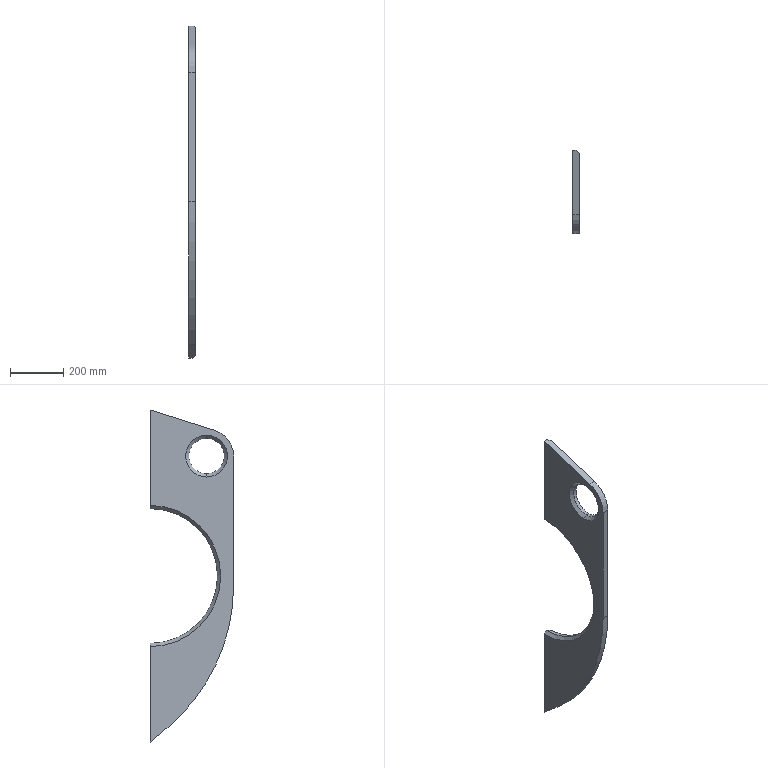Part | SolidWorks | features Chamfer 2, Extrusion 1, Fillet 1, ICE 1 | 1 solid | 17 faces | box 25 x 312.3 x 1246 mm | volume 4938572 mm3 | plane 9 | cylinder 5 | cone 3 | commonest cylinder face diameters 133 x2 203 x1 506 x1 1400 x1
STEP:
#1=CARTESIAN_POINT('',(-0.5,-212.,383.5));
#2=VERTEX_POINT('',#1);
#3=CARTESIAN_POINT('',(-0.5,-212.,516.5));
#4=VERTEX_POINT('',#3);
#5=CARTESIAN_POINT('',(-0.5,-212.,450.));
#6=DIRECTION('',(-1.,0.,0.));
#7=DIRECTION('',(0.,0.,-1.));
#8=AXIS2_PLACEMENT_3D('',#5,#6,#7);
#9=CIRCLE('',#8,66.5);
#10=EDGE_CURVE('',#2,#4,#9,.T.);
#11=ORIENTED_EDGE('',*,*,#10,.F.);
#12=CARTESIAN_POINT('',(-12.5,-212.,371.5));
#13=VERTEX_POINT('',#12);
#14=CARTESIAN_POINT('',(-12.5,-212.,371.5));
#15=DIRECTION('',(-0.7071,0.,-0.7071));
#16=VECTOR('',#15,1000.);
#17=LINE('',#14,#16);
#18=EDGE_CURVE('',#2,#13,#17,.T.);
#19=ORIENTED_EDGE('',*,*,#18,.T.);
#20=CARTESIAN_POINT('',(-12.5,-212.,528.5));
#21=VERTEX_POINT('',#20);
#22=CARTESIAN_POINT('',(-12.5,-212.,450.));
#23=DIRECTION('',(1.,0.,0.));
#24=DIRECTION('',(0.,0.,-1.));
#25=AXIS2_PLACEMENT_3D('',#22,#23,#24);
#26=CIRCLE('',#25,78.5);
#27=EDGE_CURVE('',#21,#13,#26,.T.);
#28=ORIENTED_EDGE('',*,*,#27,.F.);
#29=CARTESIAN_POINT('',(-12.5,-212.,528.5));
#30=DIRECTION('',(-0.7071,0.,0.7071));
#31=VECTOR('',#30,1000.);
#32=LINE('',#29,#31);
#33=EDGE_CURVE('',#4,#21,#32,.T.);
#34=ORIENTED_EDGE('',*,*,#33,.F.);
#35=EDGE_LOOP('',(#11,#19,#28,#34));
#36=FACE_OUTER_BOUND('',#35,.T.);
#37=CARTESIAN_POINT('',(-12.5,-212.,450.));
#38=DIRECTION('',(-1.,0.,0.));
#39=DIRECTION('',(0.,0.,1.));
#40=AXIS2_PLACEMENT_3D('',#37,#38,#39);
#41=CONICAL_SURFACE('',#40,78.5,0.7854);
#42=ADVANCED_FACE('',(#36),#41,.F.);
#43=ORIENTED_EDGE('',*,*,#10,.T.);
#44=CARTESIAN_POINT('',(12.5,-212.,516.5));
#45=VERTEX_POINT('',#44);
#46=CARTESIAN_POINT('',(-12.5,-212.,516.5));
#47=DIRECTION('',(1.,0.,0.));
#48=VECTOR('',#47,1000.);
#49=LINE('',#46,#48);
#50=EDGE_CURVE('',#4,#45,#49,.T.);
#51=ORIENTED_EDGE('',*,*,#50,.T.);
#52=CARTESIAN_POINT('',(12.5,-212.,383.5));
#53=VERTEX_POINT('',#52);
#54=CARTESIAN_POINT('',(12.5,-212.,450.));
#55=DIRECTION('',(1.,0.,0.));
#56=DIRECTION('',(0.,0.,-1.));
#57=AXIS2_PLACEMENT_3D('',#54,#55,#56);
#58=CIRCLE('',#57,66.5);
#59=EDGE_CURVE('',#45,#53,#58,.T.);
#60=ORIENTED_EDGE('',*,*,#59,.T.);
#61=CARTESIAN_POINT('',(-12.5,-212.,383.5));
#62=DIRECTION('',(1.,0.,0.));
#63=VECTOR('',#62,1000.);
#64=LINE('',#61,#63);
#65=EDGE_CURVE('',#2,#53,#64,.T.);
#66=ORIENTED_EDGE('',*,*,#65,.F.);
#67=EDGE_LOOP('',(#43,#51,#60,#66));
#68=FACE_OUTER_BOUND('',#67,.T.);
#69=CARTESIAN_POINT('',(-12.5,-212.,450.));
#70=DIRECTION('',(1.,0.,0.));
#71=DIRECTION('',(0.,0.,-1.));
#72=AXIS2_PLACEMENT_3D('',#69,#70,#71);
#73=CYLINDRICAL_SURFACE('',#72,66.5);
#74=ADVANCED_FACE('',(#68),#73,.F.);
#75=CARTESIAN_POINT('',(12.5,-13.2,-252.655));
#76=VERTEX_POINT('',#75);
#77=CARTESIAN_POINT('',(12.5,-13.2,252.655));
#78=VERTEX_POINT('',#77);
#79=CARTESIAN_POINT('',(12.5,0.,0.));
#80=DIRECTION('',(-1.,0.,0.));
#81=DIRECTION('',(0.,0.,-1.));
#82=AXIS2_PLACEMENT_3D('',#79,#80,#81);
#83=CIRCLE('',#82,253.);
#84=EDGE_CURVE('',#76,#78,#83,.T.);
#85=ORIENTED_EDGE('',*,*,#84,.F.);
#86=CARTESIAN_POINT('',(0.5,-1.2,-252.997));
#87=VERTEX_POINT('',#86);
#88=CARTESIAN_POINT('',(12.5,-13.2,-252.655));
#89=CARTESIAN_POINT('',(8.503,-9.203,-252.864));
#90=CARTESIAN_POINT('',(4.502,-5.202,-252.978));
#91=CARTESIAN_POINT('',(0.5,-1.2,-252.997));
#92=(BOUNDED_CURVE()B_SPLINE_CURVE(3,(#88,#89,#90,#91),.UNSPECIFIED.,.F.,.F.)B_SPLINE_CURVE_WITH_KNOTS((4,4),(4.66,4.708),.UNSPECIFIED.)CURVE()GEOMETRIC_REPRESENTATION_ITEM()RATIONAL_B_SPLINE_CURVE((1.,0.9998,0.9998,1.))REPRESENTATION_ITEM(''));
#93=EDGE_CURVE('',#76,#87,#92,.T.);
#94=ORIENTED_EDGE('',*,*,#93,.T.);
#95=CARTESIAN_POINT('',(-0.5,-1.2,-252.997));
#96=VERTEX_POINT('',#95);
#97=CARTESIAN_POINT('',(12.5,-1.2,-252.997));
#98=DIRECTION('',(-1.,0.,0.));
#99=VECTOR('',#98,1000.);
#100=LINE('',#97,#99);
#101=EDGE_CURVE('',#87,#96,#100,.T.);
#102=ORIENTED_EDGE('',*,*,#101,.T.);
#103=CARTESIAN_POINT('',(-0.5,-1.2,252.997));
#104=VERTEX_POINT('',#103);
#105=CARTESIAN_POINT('',(-0.5,0.,0.));
#106=DIRECTION('',(-1.,0.,0.));
#107=DIRECTION('',(0.,0.,-1.));
#108=AXIS2_PLACEMENT_3D('',#105,#106,#107);
#109=CIRCLE('',#108,253.);
#110=EDGE_CURVE('',#96,#104,#109,.T.);
#111=ORIENTED_EDGE('',*,*,#110,.T.);
#112=CARTESIAN_POINT('',(0.5,-1.2,252.997));
#113=VERTEX_POINT('',#112);
#114=CARTESIAN_POINT('',(12.5,-1.2,252.997));
#115=DIRECTION('',(-1.,0.,0.));
#116=VECTOR('',#115,1000.);
#117=LINE('',#114,#116);
#118=EDGE_CURVE('',#113,#104,#117,.T.);
#119=ORIENTED_EDGE('',*,*,#118,.F.);
#120=CARTESIAN_POINT('',(0.5,-1.2,252.997));
#121=CARTESIAN_POINT('',(4.502,-5.202,252.978));
#122=CARTESIAN_POINT('',(8.503,-9.203,252.864));
#123=CARTESIAN_POINT('',(12.5,-13.2,252.655));
#124=(BOUNDED_CURVE()B_SPLINE_CURVE(3,(#120,#121,#122,#123),.UNSPECIFIED.,.F.,.F.)B_SPLINE_CURVE_WITH_KNOTS((4,4),(1.576,1.623),.UNSPECIFIED.)CURVE()GEOMETRIC_REPRESENTATION_ITEM()RATIONAL_B_SPLINE_CURVE((1.,0.9998,0.9998,1.))REPRESENTATION_ITEM(''));
#125=EDGE_CURVE('',#113,#78,#124,.T.);
#126=ORIENTED_EDGE('',*,*,#125,.T.);
#127=EDGE_LOOP('',(#85,#94,#102,#111,#119,#126));
#128=FACE_OUTER_BOUND('',#127,.T.);
#129=CARTESIAN_POINT('',(12.5,0.,0.));
#130=DIRECTION('',(-1.,0.,0.));
#131=DIRECTION('',(0.,0.,1.));
#132=AXIS2_PLACEMENT_3D('',#129,#130,#131);
#133=CYLINDRICAL_SURFACE('',#132,253.);
#134=ADVANCED_FACE('',(#128),#133,.F.);
#135=CARTESIAN_POINT('',(0.5,-1.2,623.));
#136=VERTEX_POINT('',#135);
#137=CARTESIAN_POINT('',(-12.5,-1.2,623.));
#138=VERTEX_POINT('',#137);
#139=CARTESIAN_POINT('',(12.5,-1.2,623.));
#140=DIRECTION('',(-1.,0.,0.));
#141=VECTOR('',#140,1000.);
#142=LINE('',#139,#141);
#143=EDGE_CURVE('',#136,#138,#142,.T.);
#144=ORIENTED_EDGE('',*,*,#143,.F.);
#145=CARTESIAN_POINT('',(0.5,-1.2,252.997));
#146=DIRECTION('',(0.,0.,-1.));
#147=VECTOR('',#146,1000.);
#148=LINE('',#145,#147);
#149=EDGE_CURVE('',#136,#113,#148,.T.);
#150=ORIENTED_EDGE('',*,*,#149,.T.);
#151=ORIENTED_EDGE('',*,*,#118,.T.);
#152=CARTESIAN_POINT('',(-12.5,-1.2,264.997));
#153=VERTEX_POINT('',#152);
#154=CARTESIAN_POINT('',(-0.5,-1.2,252.997));
#155=CARTESIAN_POINT('',(-4.5,-1.2,256.997));
#156=CARTESIAN_POINT('',(-8.5,-1.2,260.997));
#157=CARTESIAN_POINT('',(-12.5,-1.2,264.997));
#158=B_SPLINE_CURVE_WITH_KNOTS('',3,(#154,#155,#156,#157),.UNSPECIFIED.,.F.,.F.,(4,4),(0.,0.01697),.UNSPECIFIED.);
#159=EDGE_CURVE('',#104,#153,#158,.T.);
#160=ORIENTED_EDGE('',*,*,#159,.T.);
#161=CARTESIAN_POINT('',(-12.5,-1.2,252.997));
#162=DIRECTION('',(0.,0.,1.));
#163=VECTOR('',#162,1000.);
#164=LINE('',#161,#163);
#165=EDGE_CURVE('',#153,#138,#164,.T.);
#166=ORIENTED_EDGE('',*,*,#165,.T.);
#167=EDGE_LOOP('',(#144,#150,#151,#160,#166));
#168=FACE_OUTER_BOUND('',#167,.T.);
#169=CARTESIAN_POINT('',(12.5,-1.2,252.997));
#170=DIRECTION('',(0.,-1.,0.));
#171=DIRECTION('',(0.,0.,-1.));
#172=AXIS2_PLACEMENT_3D('',#169,#170,#171);
#173=PLANE('',#172);
#174=ADVANCED_FACE('',(#168),#173,.F.);
#175=CARTESIAN_POINT('',(12.5,-13.2,619.211));
#176=VERTEX_POINT('',#175);
#177=CARTESIAN_POINT('',(12.5,-242.562,546.79));
#178=VERTEX_POINT('',#177);
#179=CARTESIAN_POINT('',(12.5,-1.2,623.));
#180=DIRECTION('',(0.,-0.9536,-0.3011));
#181=VECTOR('',#180,1000.);
#182=LINE('',#179,#181);
#183=EDGE_CURVE('',#176,#178,#182,.T.);
#184=ORIENTED_EDGE('',*,*,#183,.F.);
#185=CARTESIAN_POINT('',(105.617,-106.317,589.809));
#186=DIRECTION('',(-0.6901,0.6901,0.2179));
#187=VECTOR('',#186,1000.);
#188=LINE('',#185,#187);
#189=EDGE_CURVE('',#176,#136,#188,.T.);
#190=ORIENTED_EDGE('',*,*,#189,.T.);
#191=ORIENTED_EDGE('',*,*,#143,.T.);
#192=CARTESIAN_POINT('',(-12.5,-242.562,546.79));
#193=VERTEX_POINT('',#192);
#194=CARTESIAN_POINT('',(-12.5,-1.2,623.));
#195=DIRECTION('',(0.,-0.9536,-0.3011));
#196=VECTOR('',#195,1000.);
#197=LINE('',#194,#196);
#198=EDGE_CURVE('',#138,#193,#197,.T.);
#199=ORIENTED_EDGE('',*,*,#198,.T.);
#200=CARTESIAN_POINT('',(12.5,-242.562,546.79));
#201=DIRECTION('',(-1.,0.,0.));
#202=VECTOR('',#201,1000.);
#203=LINE('',#200,#202);
#204=EDGE_CURVE('',#178,#193,#203,.T.);
#205=ORIENTED_EDGE('',*,*,#204,.F.);
#206=EDGE_LOOP('',(#184,#190,#191,#199,#205));
#207=FACE_OUTER_BOUND('',#206,.T.);
#208=CARTESIAN_POINT('',(12.5,-1.2,623.));
#209=DIRECTION('',(0.,0.3011,-0.9536));
#210=DIRECTION('',(0.,0.9536,0.3011));
#211=AXIS2_PLACEMENT_3D('',#208,#209,#210);
#212=PLANE('',#211);
#213=ADVANCED_FACE('',(#207),#212,.F.);
#214=CARTESIAN_POINT('',(-12.5,-313.5,450.));
#215=VERTEX_POINT('',#214);
#216=CARTESIAN_POINT('',(-12.5,-212.,450.));
#217=DIRECTION('',(1.,0.,0.));
#218=DIRECTION('',(0.,0.,-1.));
#219=AXIS2_PLACEMENT_3D('',#216,#217,#218);
#220=CIRCLE('',#219,101.5);
#221=EDGE_CURVE('',#193,#215,#220,.T.);
#222=ORIENTED_EDGE('',*,*,#221,.T.);
#223=CARTESIAN_POINT('',(12.5,-313.5,450.));
#224=VERTEX_POINT('',#223);
#225=CARTESIAN_POINT('',(12.5,-313.5,450.));
#226=DIRECTION('',(-1.,0.,0.));
#227=VECTOR('',#226,1000.);
#228=LINE('',#225,#227);
#229=EDGE_CURVE('',#224,#215,#228,.T.);
#230=ORIENTED_EDGE('',*,*,#229,.F.);
#231=CARTESIAN_POINT('',(12.5,-212.,450.));
#232=DIRECTION('',(1.,0.,0.));
#233=DIRECTION('',(0.,0.,-1.));
#234=AXIS2_PLACEMENT_3D('',#231,#232,#233);
#235=CIRCLE('',#234,101.5);
#236=EDGE_CURVE('',#178,#224,#235,.T.);
#237=ORIENTED_EDGE('',*,*,#236,.F.);
#238=ORIENTED_EDGE('',*,*,#204,.T.);
#239=EDGE_LOOP('',(#222,#230,#237,#238));
#240=FACE_OUTER_BOUND('',#239,.T.);
#241=CARTESIAN_POINT('',(12.5,-212.,450.));
#242=DIRECTION('',(-1.,0.,0.));
#243=DIRECTION('',(0.,0.,1.));
#244=AXIS2_PLACEMENT_3D('',#241,#242,#243);
#245=CYLINDRICAL_SURFACE('',#244,101.5);
#246=ADVANCED_FACE('',(#240),#245,.T.);
#247=CARTESIAN_POINT('',(-12.5,-313.5,-34.534));
#248=VERTEX_POINT('',#247);
#249=CARTESIAN_POINT('',(-12.5,-313.5,450.));
#250=DIRECTION('',(0.,0.,-1.));
#251=VECTOR('',#250,1000.);
#252=LINE('',#249,#251);
#253=EDGE_CURVE('',#215,#248,#252,.T.);
#254=ORIENTED_EDGE('',*,*,#253,.T.);
#255=CARTESIAN_POINT('',(12.5,-313.5,-34.534));
#256=VERTEX_POINT('',#255);
#257=CARTESIAN_POINT('',(12.5,-313.5,-34.534));
#258=DIRECTION('',(1.,0.,0.));
#259=VECTOR('',#258,1000.);
#260=LINE('',#257,#259);
#261=EDGE_CURVE('',#248,#256,#260,.T.);
#262=ORIENTED_EDGE('',*,*,#261,.T.);
#263=CARTESIAN_POINT('',(12.5,-313.5,450.));
#264=DIRECTION('',(0.,0.,-1.));
#265=VECTOR('',#264,1000.);
#266=LINE('',#263,#265);
#267=EDGE_CURVE('',#224,#256,#266,.T.);
#268=ORIENTED_EDGE('',*,*,#267,.F.);
#269=ORIENTED_EDGE('',*,*,#229,.T.);
#270=EDGE_LOOP('',(#254,#262,#268,#269));
#271=FACE_OUTER_BOUND('',#270,.T.);
#272=CARTESIAN_POINT('',(12.5,-313.5,450.));
#273=DIRECTION('',(0.,1.,0.));
#274=DIRECTION('',(0.,0.,1.));
#275=AXIS2_PLACEMENT_3D('',#272,#273,#274);
#276=PLANE('',#275);
#277=ADVANCED_FACE('',(#271),#276,.F.);
#278=CARTESIAN_POINT('',(0.5,-1.2,-623.));
#279=VERTEX_POINT('',#278);
#280=CARTESIAN_POINT('',(-12.5,-1.2,-623.));
#281=VERTEX_POINT('',#280);
#282=CARTESIAN_POINT('',(12.5,-1.2,-623.));
#283=DIRECTION('',(-1.,0.,0.));
#284=VECTOR('',#283,1000.);
#285=LINE('',#282,#284);
#286=EDGE_CURVE('',#279,#281,#285,.T.);
#287=ORIENTED_EDGE('',*,*,#286,.F.);
#288=CARTESIAN_POINT('',(12.5,-13.2,-612.931));
#289=VERTEX_POINT('',#288);
#290=CARTESIAN_POINT('',(202.697,-203.397,-453.336));
#291=DIRECTION('',(0.6081,-0.6081,0.5103));
#292=VECTOR('',#291,1000.);
#293=LINE('',#290,#292);
#294=EDGE_CURVE('',#279,#289,#293,.T.);
#295=ORIENTED_EDGE('',*,*,#294,.T.);
#296=CARTESIAN_POINT('',(12.5,-63.451,-570.765));
#297=VERTEX_POINT('',#296);
#298=CARTESIAN_POINT('',(12.5,-313.5,-360.949));
#299=DIRECTION('',(0.,0.766,-0.6428));
#300=VECTOR('',#299,1000.);
#301=LINE('',#298,#300);
#302=EDGE_CURVE('',#297,#289,#301,.T.);
#303=ORIENTED_EDGE('',*,*,#302,.F.);
#304=CARTESIAN_POINT('',(-12.5,-63.451,-570.765));
#305=VERTEX_POINT('',#304);
#306=CARTESIAN_POINT('',(12.5,-63.451,-570.765));
#307=DIRECTION('',(-1.,0.,0.));
#308=VECTOR('',#307,1000.);
#309=LINE('',#306,#308);
#310=EDGE_CURVE('',#297,#305,#309,.T.);
#311=ORIENTED_EDGE('',*,*,#310,.T.);
#312=CARTESIAN_POINT('',(-12.5,-313.5,-360.949));
#313=DIRECTION('',(0.,0.766,-0.6428));
#314=VECTOR('',#313,1000.);
#315=LINE('',#312,#314);
#316=EDGE_CURVE('',#305,#281,#315,.T.);
#317=ORIENTED_EDGE('',*,*,#316,.T.);
#318=EDGE_LOOP('',(#287,#295,#303,#311,#317));
#319=FACE_OUTER_BOUND('',#318,.T.);
#320=CARTESIAN_POINT('',(12.5,-313.5,-360.949));
#321=DIRECTION('',(0.,0.6428,0.766));
#322=DIRECTION('',(0.,-0.766,0.6428));
#323=AXIS2_PLACEMENT_3D('',#320,#321,#322);
#324=PLANE('',#323);
#325=ADVANCED_FACE('',(#319),#324,.F.);
#326=ORIENTED_EDGE('',*,*,#101,.F.);
#327=CARTESIAN_POINT('',(0.5,-1.2,-623.));
#328=DIRECTION('',(0.,0.,-1.));
#329=VECTOR('',#328,1000.);
#330=LINE('',#327,#329);
#331=EDGE_CURVE('',#87,#279,#330,.T.);
#332=ORIENTED_EDGE('',*,*,#331,.T.);
#333=ORIENTED_EDGE('',*,*,#286,.T.);
#334=CARTESIAN_POINT('',(-12.5,-1.2,-264.997));
#335=VERTEX_POINT('',#334);
#336=CARTESIAN_POINT('',(-12.5,-1.2,-623.));
#337=DIRECTION('',(0.,0.,1.));
#338=VECTOR('',#337,1000.);
#339=LINE('',#336,#338);
#340=EDGE_CURVE('',#281,#335,#339,.T.);
#341=ORIENTED_EDGE('',*,*,#340,.T.);
#342=CARTESIAN_POINT('',(-12.5,-1.2,-264.997));
#343=CARTESIAN_POINT('',(-8.5,-1.2,-260.997));
#344=CARTESIAN_POINT('',(-4.5,-1.2,-256.997));
#345=CARTESIAN_POINT('',(-0.5,-1.2,-252.997));
#346=B_SPLINE_CURVE_WITH_KNOTS('',3,(#342,#343,#344,#345),.UNSPECIFIED.,.F.,.F.,(4,4),(0.,0.01697),.UNSPECIFIED.);
#347=EDGE_CURVE('',#335,#96,#346,.T.);
#348=ORIENTED_EDGE('',*,*,#347,.T.);
#349=EDGE_LOOP('',(#326,#332,#333,#341,#348));
#350=FACE_OUTER_BOUND('',#349,.T.);
#351=CARTESIAN_POINT('',(12.5,-1.2,-623.));
#352=DIRECTION('',(0.,-1.,0.));
#353=DIRECTION('',(0.,0.,-1.));
#354=AXIS2_PLACEMENT_3D('',#351,#352,#353);
#355=PLANE('',#354);
#356=ADVANCED_FACE('',(#350),#355,.F.);
#357=CARTESIAN_POINT('',(12.5,-212.,450.));
#358=DIRECTION('',(1.,0.,0.));
#359=DIRECTION('',(0.,0.,-1.));
#360=AXIS2_PLACEMENT_3D('',#357,#358,#359);
#361=CIRCLE('',#360,66.5);
#362=EDGE_CURVE('',#53,#45,#361,.T.);
#363=ORIENTED_EDGE('',*,*,#362,.F.);
#364=ORIENTED_EDGE('',*,*,#59,.F.);
#365=EDGE_LOOP('',(#363,#364));
#366=FACE_BOUND('',#365,.T.);
#367=ORIENTED_EDGE('',*,*,#302,.T.);
#368=CARTESIAN_POINT('',(12.5,-13.2,-252.997));
#369=DIRECTION('',(0.,0.,1.));
#370=VECTOR('',#369,1000.);
#371=LINE('',#368,#370);
#372=EDGE_CURVE('',#289,#76,#371,.T.);
#373=ORIENTED_EDGE('',*,*,#372,.T.);
#374=ORIENTED_EDGE('',*,*,#84,.T.);
#375=CARTESIAN_POINT('',(12.5,-13.2,623.));
#376=DIRECTION('',(0.,0.,1.));
#377=VECTOR('',#376,1000.);
#378=LINE('',#375,#377);
#379=EDGE_CURVE('',#78,#176,#378,.T.);
#380=ORIENTED_EDGE('',*,*,#379,.T.);
#381=ORIENTED_EDGE('',*,*,#183,.T.);
#382=ORIENTED_EDGE('',*,*,#236,.T.);
#383=ORIENTED_EDGE('',*,*,#267,.T.);
#384=CARTESIAN_POINT('',(12.5,386.5,-34.534));
#385=DIRECTION('',(1.,0.,0.));
#386=DIRECTION('',(0.,0.,-1.));
#387=AXIS2_PLACEMENT_3D('',#384,#385,#386);
#388=CIRCLE('',#387,700.);
#389=EDGE_CURVE('',#256,#297,#388,.T.);
#390=ORIENTED_EDGE('',*,*,#389,.T.);
#391=EDGE_LOOP('',(#367,#373,#374,#380,#381,#382,#383,#390));
#392=FACE_OUTER_BOUND('',#391,.T.);
#393=CARTESIAN_POINT('',(12.5,0.,0.));
#394=DIRECTION('',(1.,0.,0.));
#395=DIRECTION('',(0.,0.,-1.));
#396=AXIS2_PLACEMENT_3D('',#393,#394,#395);
#397=PLANE('',#396);
#398=ADVANCED_FACE('',(#366,#392),#397,.T.);
#399=ORIENTED_EDGE('',*,*,#27,.T.);
#400=CARTESIAN_POINT('',(-12.5,-212.,450.));
#401=DIRECTION('',(1.,0.,0.));
#402=DIRECTION('',(0.,0.,-1.));
#403=AXIS2_PLACEMENT_3D('',#400,#401,#402);
#404=CIRCLE('',#403,78.5);
#405=EDGE_CURVE('',#13,#21,#404,.T.);
#406=ORIENTED_EDGE('',*,*,#405,.T.);
#407=EDGE_LOOP('',(#399,#406));
#408=FACE_BOUND('',#407,.T.);
#409=ORIENTED_EDGE('',*,*,#165,.F.);
#410=CARTESIAN_POINT('',(-12.5,0.,0.));
#411=DIRECTION('',(1.,0.,0.));
#412=DIRECTION('',(0.,0.,-1.));
#413=AXIS2_PLACEMENT_3D('',#410,#411,#412);
#414=CIRCLE('',#413,265.);
#415=EDGE_CURVE('',#153,#335,#414,.T.);
#416=ORIENTED_EDGE('',*,*,#415,.T.);
#417=ORIENTED_EDGE('',*,*,#340,.F.);
#418=ORIENTED_EDGE('',*,*,#316,.F.);
#419=CARTESIAN_POINT('',(-12.5,386.5,-34.534));
#420=DIRECTION('',(-1.,0.,0.));
#421=DIRECTION('',(0.,0.,-1.));
#422=AXIS2_PLACEMENT_3D('',#419,#420,#421);
#423=CIRCLE('',#422,700.);
#424=EDGE_CURVE('',#305,#248,#423,.T.);
#425=ORIENTED_EDGE('',*,*,#424,.T.);
#426=ORIENTED_EDGE('',*,*,#253,.F.);
#427=ORIENTED_EDGE('',*,*,#221,.F.);
#428=ORIENTED_EDGE('',*,*,#198,.F.);
#429=EDGE_LOOP('',(#409,#416,#417,#418,#425,#426,#427,#428));
#430=FACE_OUTER_BOUND('',#429,.T.);
#431=CARTESIAN_POINT('',(-12.5,0.,0.));
#432=DIRECTION('',(1.,0.,0.));
#433=DIRECTION('',(0.,0.,-1.));
#434=AXIS2_PLACEMENT_3D('',#431,#432,#433);
#435=PLANE('',#434);
#436=ADVANCED_FACE('',(#408,#430),#435,.F.);
#437=ORIENTED_EDGE('',*,*,#50,.F.);
#438=CARTESIAN_POINT('',(-0.5,-212.,450.));
#439=DIRECTION('',(-1.,0.,0.));
#440=DIRECTION('',(0.,0.,-1.));
#441=AXIS2_PLACEMENT_3D('',#438,#439,#440);
#442=CIRCLE('',#441,66.5);
#443=EDGE_CURVE('',#4,#2,#442,.T.);
#444=ORIENTED_EDGE('',*,*,#443,.T.);
#445=ORIENTED_EDGE('',*,*,#65,.T.);
#446=ORIENTED_EDGE('',*,*,#362,.T.);
#447=EDGE_LOOP('',(#437,#444,#445,#446));
#448=FACE_OUTER_BOUND('',#447,.T.);
#449=CARTESIAN_POINT('',(-12.5,-212.,450.));
#450=DIRECTION('',(1.,0.,0.));
#451=DIRECTION('',(0.,0.,-1.));
#452=AXIS2_PLACEMENT_3D('',#449,#450,#451);
#453=CYLINDRICAL_SURFACE('',#452,66.5);
#454=ADVANCED_FACE('',(#448),#453,.F.);
#455=ORIENTED_EDGE('',*,*,#389,.F.);
#456=ORIENTED_EDGE('',*,*,#261,.F.);
#457=ORIENTED_EDGE('',*,*,#424,.F.);
#458=ORIENTED_EDGE('',*,*,#310,.F.);
#459=EDGE_LOOP('',(#455,#456,#457,#458));
#460=FACE_OUTER_BOUND('',#459,.T.);
#461=CARTESIAN_POINT('',(12.5,386.5,-34.534));
#462=DIRECTION('',(-1.,0.,0.));
#463=DIRECTION('',(0.,0.,1.));
#464=AXIS2_PLACEMENT_3D('',#461,#462,#463);
#465=CYLINDRICAL_SURFACE('',#464,700.);
#466=ADVANCED_FACE('',(#460),#465,.T.);
#467=ORIENTED_EDGE('',*,*,#18,.F.);
#468=ORIENTED_EDGE('',*,*,#443,.F.);
#469=ORIENTED_EDGE('',*,*,#33,.T.);
#470=ORIENTED_EDGE('',*,*,#405,.F.);
#471=EDGE_LOOP('',(#467,#468,#469,#470));
#472=FACE_OUTER_BOUND('',#471,.T.);
#473=CARTESIAN_POINT('',(-12.5,-212.,450.));
#474=DIRECTION('',(-1.,0.,0.));
#475=DIRECTION('',(0.,0.,1.));
#476=AXIS2_PLACEMENT_3D('',#473,#474,#475);
#477=CONICAL_SURFACE('',#476,78.5,0.7854);
#478=ADVANCED_FACE('',(#472),#477,.F.);
#479=ORIENTED_EDGE('',*,*,#347,.F.);
#480=ORIENTED_EDGE('',*,*,#415,.F.);
#481=ORIENTED_EDGE('',*,*,#159,.F.);
#482=ORIENTED_EDGE('',*,*,#110,.F.);
#483=EDGE_LOOP('',(#479,#480,#481,#482));
#484=FACE_OUTER_BOUND('',#483,.T.);
#485=CARTESIAN_POINT('',(-0.5,0.,0.));
#486=DIRECTION('',(-1.,0.,0.));
#487=DIRECTION('',(0.,0.,1.));
#488=AXIS2_PLACEMENT_3D('',#485,#486,#487);
#489=CONICAL_SURFACE('',#488,253.,0.7854);
#490=ADVANCED_FACE('',(#484),#489,.F.);
#491=ORIENTED_EDGE('',*,*,#294,.F.);
#492=ORIENTED_EDGE('',*,*,#331,.F.);
#493=ORIENTED_EDGE('',*,*,#93,.F.);
#494=ORIENTED_EDGE('',*,*,#372,.F.);
#495=EDGE_LOOP('',(#491,#492,#493,#494));
#496=FACE_OUTER_BOUND('',#495,.T.);
#497=CARTESIAN_POINT('',(12.5,-13.2,0.));
#498=DIRECTION('',(0.7071,0.7071,0.));
#499=DIRECTION('',(0.,0.,-1.));
#500=AXIS2_PLACEMENT_3D('',#497,#498,#499);
#501=PLANE('',#500);
#502=ADVANCED_FACE('',(#496),#501,.T.);
#503=ORIENTED_EDGE('',*,*,#125,.F.);
#504=ORIENTED_EDGE('',*,*,#149,.F.);
#505=ORIENTED_EDGE('',*,*,#189,.F.);
#506=ORIENTED_EDGE('',*,*,#379,.F.);
#507=EDGE_LOOP('',(#503,#504,#505,#506));
#508=FACE_OUTER_BOUND('',#507,.T.);
#509=CARTESIAN_POINT('',(12.5,-13.2,0.));
#510=DIRECTION('',(0.7071,0.7071,0.));
#511=DIRECTION('',(0.,0.,-1.));
#512=AXIS2_PLACEMENT_3D('',#509,#510,#511);
#513=PLANE('',#512);
#514=ADVANCED_FACE('',(#508),#513,.T.);
#515=CLOSED_SHELL('',(#42,#74,#134,#174,#213,#246,#277,#325,#356,#398,#436,#454,#466,#478,#490,#502,#514));
#516=MANIFOLD_SOLID_BREP('',#515);
#517=CARTESIAN_POINT('',(0.,0.,0.));
#518=DIRECTION('',(0.,0.,1.));
#519=DIRECTION('',(1.,0.,0.));
#520=AXIS2_PLACEMENT_3D('',#517,#518,#519);
#521=(LENGTH_UNIT()NAMED_UNIT(*)SI_UNIT(.MILLI.,.METRE.));
#522=UNCERTAINTY_MEASURE_WITH_UNIT(LENGTH_MEASURE(0.00001),#521,'','');
#523=(NAMED_UNIT(*)PLANE_ANGLE_UNIT()SI_UNIT($,.RADIAN.));
#524=(NAMED_UNIT(*)SI_UNIT($,.STERADIAN.)SOLID_ANGLE_UNIT());
#525=(GEOMETRIC_REPRESENTATION_CONTEXT(3)GLOBAL_UNCERTAINTY_ASSIGNED_CONTEXT((#522))GLOBAL_UNIT_ASSIGNED_CONTEXT((#521,#523,#524))REPRESENTATION_CONTEXT('',''));
#526=ADVANCED_BREP_SHAPE_REPRESENTATION('',(#516,#520),#525);